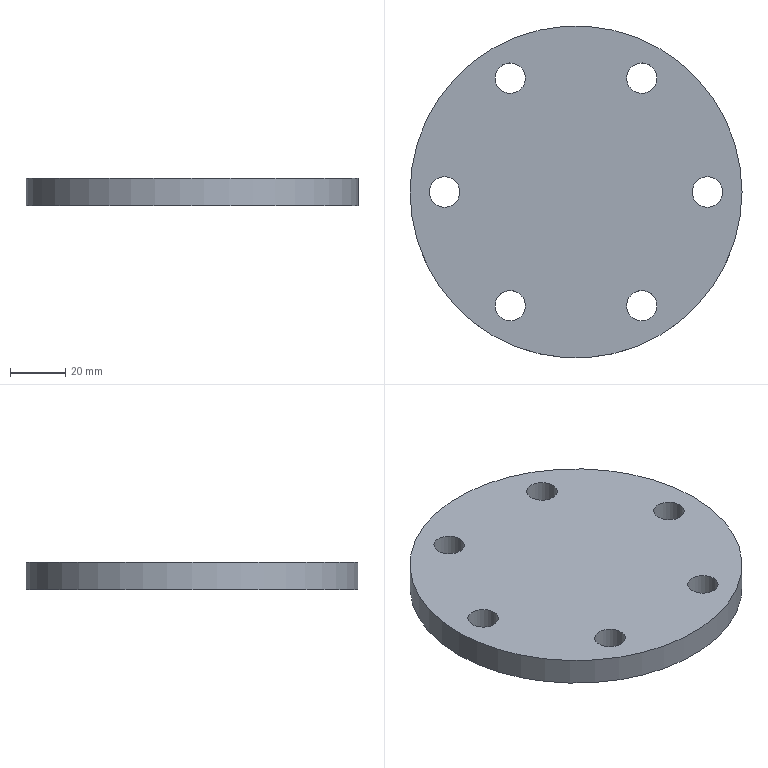Part | NX | 1 solid | 9 faces | box 120 x 120 x 10 mm | volume 107395 mm3 | cylinder 7 | plane 2 | commonest cylinder face diameters 11 x6 120 x1
STEP:
#1=CARTESIAN_POINT('',(2995.931,208.53,-928.));
#2=VERTEX_POINT('',#1);
#3=CARTESIAN_POINT('',(2998.681,203.767,-928.));
#4=DIRECTION('',(0.,0.,-1.));
#5=DIRECTION('',(-0.5,0.866,0.));
#6=AXIS2_PLACEMENT_3D('',#3,#4,#5);
#7=CIRCLE('',#6,5.5);
#8=EDGE_CURVE('',#2,#2,#7,.T.);
#9=ORIENTED_EDGE('',*,*,#8,.T.);
#10=EDGE_LOOP('',(#9));
#11=FACE_BOUND('',#10,.T.);
#12=CARTESIAN_POINT('',(2995.931,208.53,-918.));
#13=VERTEX_POINT('',#12);
#14=CARTESIAN_POINT('',(2998.681,203.767,-918.));
#15=DIRECTION('',(0.,0.,-1.));
#16=DIRECTION('',(-0.5,0.866,0.));
#17=AXIS2_PLACEMENT_3D('',#14,#15,#16);
#18=CIRCLE('',#17,5.5);
#19=EDGE_CURVE('',#13,#13,#18,.T.);
#20=ORIENTED_EDGE('',*,*,#19,.F.);
#21=EDGE_LOOP('',(#20));
#22=FACE_BOUND('',#21,.T.);
#23=CARTESIAN_POINT('',(2998.681,203.767,-928.));
#24=DIRECTION('',(0.,0.,1.));
#25=DIRECTION('',(-1.,0.,0.));
#26=AXIS2_PLACEMENT_3D('',#23,#24,#25);
#27=CYLINDRICAL_SURFACE('',#26,5.5);
#28=ADVANCED_FACE('',(#11,#22),#27,.F.);
#29=CARTESIAN_POINT('',(2953.931,208.53,-928.));
#30=VERTEX_POINT('',#29);
#31=CARTESIAN_POINT('',(2951.181,203.767,-928.));
#32=DIRECTION('',(0.,0.,-1.));
#33=DIRECTION('',(0.5,0.866,0.));
#34=AXIS2_PLACEMENT_3D('',#31,#32,#33);
#35=CIRCLE('',#34,5.5);
#36=EDGE_CURVE('',#30,#30,#35,.T.);
#37=ORIENTED_EDGE('',*,*,#36,.T.);
#38=EDGE_LOOP('',(#37));
#39=FACE_BOUND('',#38,.T.);
#40=CARTESIAN_POINT('',(2953.931,208.53,-918.));
#41=VERTEX_POINT('',#40);
#42=CARTESIAN_POINT('',(2951.181,203.767,-918.));
#43=DIRECTION('',(0.,0.,-1.));
#44=DIRECTION('',(0.5,0.866,0.));
#45=AXIS2_PLACEMENT_3D('',#42,#43,#44);
#46=CIRCLE('',#45,5.5);
#47=EDGE_CURVE('',#41,#41,#46,.T.);
#48=ORIENTED_EDGE('',*,*,#47,.F.);
#49=EDGE_LOOP('',(#48));
#50=FACE_BOUND('',#49,.T.);
#51=CARTESIAN_POINT('',(2951.181,203.767,-928.));
#52=DIRECTION('',(0.,0.,1.));
#53=DIRECTION('',(-1.,0.,0.));
#54=AXIS2_PLACEMENT_3D('',#51,#52,#53);
#55=CYLINDRICAL_SURFACE('',#54,5.5);
#56=ADVANCED_FACE('',(#39,#50),#55,.F.);
#57=CARTESIAN_POINT('',(2932.931,244.903,-928.));
#58=VERTEX_POINT('',#57);
#59=CARTESIAN_POINT('',(2927.431,244.903,-928.));
#60=DIRECTION('',(0.,0.,-1.));
#61=DIRECTION('',(1.,0.,0.));
#62=AXIS2_PLACEMENT_3D('',#59,#60,#61);
#63=CIRCLE('',#62,5.5);
#64=EDGE_CURVE('',#58,#58,#63,.T.);
#65=ORIENTED_EDGE('',*,*,#64,.T.);
#66=EDGE_LOOP('',(#65));
#67=FACE_BOUND('',#66,.T.);
#68=CARTESIAN_POINT('',(2932.931,244.903,-918.));
#69=VERTEX_POINT('',#68);
#70=CARTESIAN_POINT('',(2927.431,244.903,-918.));
#71=DIRECTION('',(0.,0.,-1.));
#72=DIRECTION('',(1.,0.,0.));
#73=AXIS2_PLACEMENT_3D('',#70,#71,#72);
#74=CIRCLE('',#73,5.5);
#75=EDGE_CURVE('',#69,#69,#74,.T.);
#76=ORIENTED_EDGE('',*,*,#75,.F.);
#77=EDGE_LOOP('',(#76));
#78=FACE_BOUND('',#77,.T.);
#79=CARTESIAN_POINT('',(2927.431,244.903,-928.));
#80=DIRECTION('',(0.,0.,1.));
#81=DIRECTION('',(-1.,0.,0.));
#82=AXIS2_PLACEMENT_3D('',#79,#80,#81);
#83=CYLINDRICAL_SURFACE('',#82,5.5);
#84=ADVANCED_FACE('',(#67,#78),#83,.F.);
#85=CARTESIAN_POINT('',(2953.931,281.276,-928.));
#86=VERTEX_POINT('',#85);
#87=CARTESIAN_POINT('',(2951.181,286.04,-928.));
#88=DIRECTION('',(0.,0.,-1.));
#89=DIRECTION('',(0.5,-0.866,0.));
#90=AXIS2_PLACEMENT_3D('',#87,#88,#89);
#91=CIRCLE('',#90,5.5);
#92=EDGE_CURVE('',#86,#86,#91,.T.);
#93=ORIENTED_EDGE('',*,*,#92,.T.);
#94=EDGE_LOOP('',(#93));
#95=FACE_BOUND('',#94,.T.);
#96=CARTESIAN_POINT('',(2953.931,281.276,-918.));
#97=VERTEX_POINT('',#96);
#98=CARTESIAN_POINT('',(2951.181,286.04,-918.));
#99=DIRECTION('',(0.,0.,-1.));
#100=DIRECTION('',(0.5,-0.866,0.));
#101=AXIS2_PLACEMENT_3D('',#98,#99,#100);
#102=CIRCLE('',#101,5.5);
#103=EDGE_CURVE('',#97,#97,#102,.T.);
#104=ORIENTED_EDGE('',*,*,#103,.F.);
#105=EDGE_LOOP('',(#104));
#106=FACE_BOUND('',#105,.T.);
#107=CARTESIAN_POINT('',(2951.181,286.04,-928.));
#108=DIRECTION('',(0.,0.,1.));
#109=DIRECTION('',(-1.,0.,0.));
#110=AXIS2_PLACEMENT_3D('',#107,#108,#109);
#111=CYLINDRICAL_SURFACE('',#110,5.5);
#112=ADVANCED_FACE('',(#95,#106),#111,.F.);
#113=CARTESIAN_POINT('',(2995.931,281.276,-928.));
#114=VERTEX_POINT('',#113);
#115=CARTESIAN_POINT('',(2998.681,286.04,-928.));
#116=DIRECTION('',(0.,0.,-1.));
#117=DIRECTION('',(-0.5,-0.866,0.));
#118=AXIS2_PLACEMENT_3D('',#115,#116,#117);
#119=CIRCLE('',#118,5.5);
#120=EDGE_CURVE('',#114,#114,#119,.T.);
#121=ORIENTED_EDGE('',*,*,#120,.T.);
#122=EDGE_LOOP('',(#121));
#123=FACE_BOUND('',#122,.T.);
#124=CARTESIAN_POINT('',(2995.931,281.276,-918.));
#125=VERTEX_POINT('',#124);
#126=CARTESIAN_POINT('',(2998.681,286.04,-918.));
#127=DIRECTION('',(0.,0.,-1.));
#128=DIRECTION('',(-0.5,-0.866,0.));
#129=AXIS2_PLACEMENT_3D('',#126,#127,#128);
#130=CIRCLE('',#129,5.5);
#131=EDGE_CURVE('',#125,#125,#130,.T.);
#132=ORIENTED_EDGE('',*,*,#131,.F.);
#133=EDGE_LOOP('',(#132));
#134=FACE_BOUND('',#133,.T.);
#135=CARTESIAN_POINT('',(2998.681,286.04,-928.));
#136=DIRECTION('',(0.,0.,1.));
#137=DIRECTION('',(-1.,0.,0.));
#138=AXIS2_PLACEMENT_3D('',#135,#136,#137);
#139=CYLINDRICAL_SURFACE('',#138,5.5);
#140=ADVANCED_FACE('',(#123,#134),#139,.F.);
#141=CARTESIAN_POINT('',(3034.931,244.903,-928.));
#142=VERTEX_POINT('',#141);
#143=CARTESIAN_POINT('',(2974.931,244.903,-928.));
#144=DIRECTION('',(0.,0.,-1.));
#145=DIRECTION('',(1.,0.,0.));
#146=AXIS2_PLACEMENT_3D('',#143,#144,#145);
#147=CIRCLE('',#146,60.);
#148=EDGE_CURVE('',#142,#142,#147,.T.);
#149=ORIENTED_EDGE('',*,*,#148,.F.);
#150=EDGE_LOOP('',(#149));
#151=FACE_BOUND('',#150,.T.);
#152=CARTESIAN_POINT('',(3034.931,244.903,-918.));
#153=VERTEX_POINT('',#152);
#154=CARTESIAN_POINT('',(2974.931,244.903,-918.));
#155=DIRECTION('',(0.,0.,-1.));
#156=DIRECTION('',(1.,0.,0.));
#157=AXIS2_PLACEMENT_3D('',#154,#155,#156);
#158=CIRCLE('',#157,60.);
#159=EDGE_CURVE('',#153,#153,#158,.T.);
#160=ORIENTED_EDGE('',*,*,#159,.T.);
#161=EDGE_LOOP('',(#160));
#162=FACE_BOUND('',#161,.T.);
#163=CARTESIAN_POINT('',(2974.931,244.903,-928.));
#164=DIRECTION('',(0.,0.,1.));
#165=DIRECTION('',(-1.,0.,0.));
#166=AXIS2_PLACEMENT_3D('',#163,#164,#165);
#167=CYLINDRICAL_SURFACE('',#166,60.);
#168=ADVANCED_FACE('',(#151,#162),#167,.T.);
#169=CARTESIAN_POINT('',(3016.931,244.903,-928.));
#170=VERTEX_POINT('',#169);
#171=CARTESIAN_POINT('',(3022.431,244.903,-928.));
#172=DIRECTION('',(0.,0.,-1.));
#173=DIRECTION('',(-1.,0.,0.));
#174=AXIS2_PLACEMENT_3D('',#171,#172,#173);
#175=CIRCLE('',#174,5.5);
#176=EDGE_CURVE('',#170,#170,#175,.T.);
#177=ORIENTED_EDGE('',*,*,#176,.T.);
#178=EDGE_LOOP('',(#177));
#179=FACE_BOUND('',#178,.T.);
#180=CARTESIAN_POINT('',(3016.931,244.903,-918.));
#181=VERTEX_POINT('',#180);
#182=CARTESIAN_POINT('',(3022.431,244.903,-918.));
#183=DIRECTION('',(0.,0.,-1.));
#184=DIRECTION('',(-1.,0.,0.));
#185=AXIS2_PLACEMENT_3D('',#182,#183,#184);
#186=CIRCLE('',#185,5.5);
#187=EDGE_CURVE('',#181,#181,#186,.T.);
#188=ORIENTED_EDGE('',*,*,#187,.F.);
#189=EDGE_LOOP('',(#188));
#190=FACE_BOUND('',#189,.T.);
#191=CARTESIAN_POINT('',(3022.431,244.903,-928.));
#192=DIRECTION('',(0.,0.,1.));
#193=DIRECTION('',(-1.,0.,0.));
#194=AXIS2_PLACEMENT_3D('',#191,#192,#193);
#195=CYLINDRICAL_SURFACE('',#194,5.5);
#196=ADVANCED_FACE('',(#179,#190),#195,.F.);
#197=ORIENTED_EDGE('',*,*,#148,.T.);
#198=EDGE_LOOP('',(#197));
#199=FACE_BOUND('',#198,.T.);
#200=ORIENTED_EDGE('',*,*,#120,.F.);
#201=EDGE_LOOP('',(#200));
#202=FACE_BOUND('',#201,.T.);
#203=ORIENTED_EDGE('',*,*,#92,.F.);
#204=EDGE_LOOP('',(#203));
#205=FACE_BOUND('',#204,.T.);
#206=ORIENTED_EDGE('',*,*,#64,.F.);
#207=EDGE_LOOP('',(#206));
#208=FACE_BOUND('',#207,.T.);
#209=ORIENTED_EDGE('',*,*,#36,.F.);
#210=EDGE_LOOP('',(#209));
#211=FACE_BOUND('',#210,.T.);
#212=ORIENTED_EDGE('',*,*,#8,.F.);
#213=EDGE_LOOP('',(#212));
#214=FACE_BOUND('',#213,.T.);
#215=ORIENTED_EDGE('',*,*,#176,.F.);
#216=EDGE_LOOP('',(#215));
#217=FACE_BOUND('',#216,.T.);
#218=CARTESIAN_POINT('',(2986.806,265.472,-928.));
#219=DIRECTION('',(0.,0.,-1.));
#220=DIRECTION('',(1.,0.,0.));
#221=AXIS2_PLACEMENT_3D('',#218,#219,#220);
#222=PLANE('',#221);
#223=ADVANCED_FACE('',(#199,#202,#205,#208,#211,#214,#217),#222,.T.);
#224=ORIENTED_EDGE('',*,*,#159,.F.);
#225=EDGE_LOOP('',(#224));
#226=FACE_BOUND('',#225,.T.);
#227=ORIENTED_EDGE('',*,*,#131,.T.);
#228=EDGE_LOOP('',(#227));
#229=FACE_BOUND('',#228,.T.);
#230=ORIENTED_EDGE('',*,*,#103,.T.);
#231=EDGE_LOOP('',(#230));
#232=FACE_BOUND('',#231,.T.);
#233=ORIENTED_EDGE('',*,*,#75,.T.);
#234=EDGE_LOOP('',(#233));
#235=FACE_BOUND('',#234,.T.);
#236=ORIENTED_EDGE('',*,*,#47,.T.);
#237=EDGE_LOOP('',(#236));
#238=FACE_BOUND('',#237,.T.);
#239=ORIENTED_EDGE('',*,*,#19,.T.);
#240=EDGE_LOOP('',(#239));
#241=FACE_BOUND('',#240,.T.);
#242=ORIENTED_EDGE('',*,*,#187,.T.);
#243=EDGE_LOOP('',(#242));
#244=FACE_BOUND('',#243,.T.);
#245=CARTESIAN_POINT('',(2986.806,265.472,-918.));
#246=DIRECTION('',(0.,0.,-1.));
#247=DIRECTION('',(1.,0.,0.));
#248=AXIS2_PLACEMENT_3D('',#245,#246,#247);
#249=PLANE('',#248);
#250=ADVANCED_FACE('',(#226,#229,#232,#235,#238,#241,#244),#249,.F.);
#251=CLOSED_SHELL('',(#28,#56,#84,#112,#140,#168,#196,#223,#250));
#252=MANIFOLD_SOLID_BREP('',#251);
#253=(LENGTH_UNIT()NAMED_UNIT(*)SI_UNIT(.MILLI.,.METRE.));
#254=UNCERTAINTY_MEASURE_WITH_UNIT(LENGTH_MEASURE(0.00002),#253,'','');
#255=(NAMED_UNIT(*)PLANE_ANGLE_UNIT()SI_UNIT($,.RADIAN.));
#256=PLANE_ANGLE_MEASURE_WITH_UNIT(PLANE_ANGLE_MEASURE(0.01745),#255);
#257=DIMENSIONAL_EXPONENTS(0.,0.,0.,0.,0.,0.,0.);
#258=(CONVERSION_BASED_UNIT('DEGREE',#256)NAMED_UNIT(#257)PLANE_ANGLE_UNIT());
#259=(NAMED_UNIT(*)SI_UNIT($,.STERADIAN.)SOLID_ANGLE_UNIT());
#260=(GEOMETRIC_REPRESENTATION_CONTEXT(3)GLOBAL_UNCERTAINTY_ASSIGNED_CONTEXT((#254))GLOBAL_UNIT_ASSIGNED_CONTEXT((#253,#258,#259))REPRESENTATION_CONTEXT('',''));
#261=ADVANCED_BREP_SHAPE_REPRESENTATION('',(#252),#260);